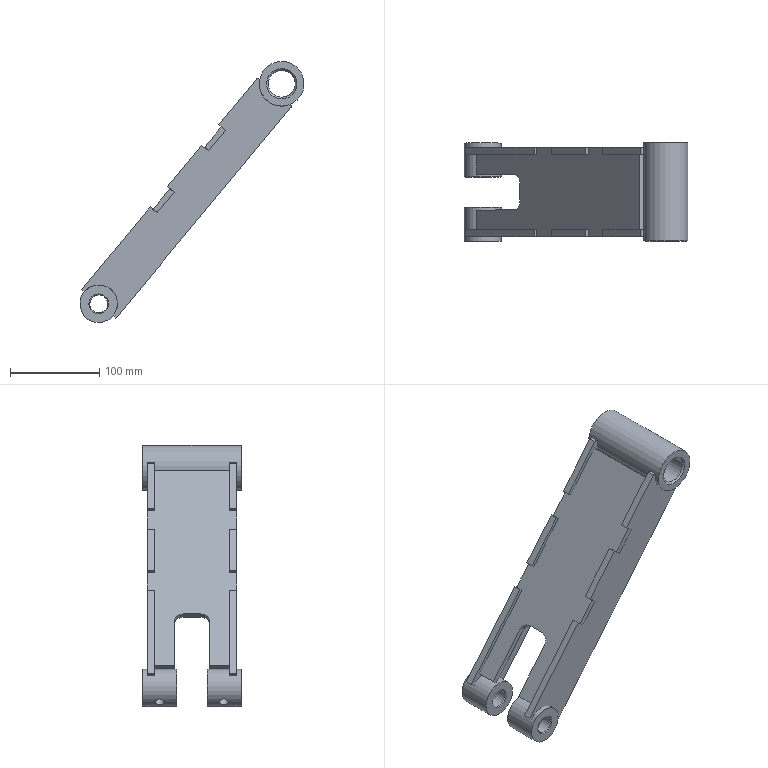Part | STEP file | HL4GZ-1.862.032 (cane-lifter upper swing arm weldment) | 7 solids | 98 faces | box 250.646 x 110 x 292.008 mm | volume 622631 mm3 | plane 70 | cylinder 22 | cone 6 | commonest cylinder face diameters 20 x6 4 x4 42 x4 50 x3 10 x2 23 x2